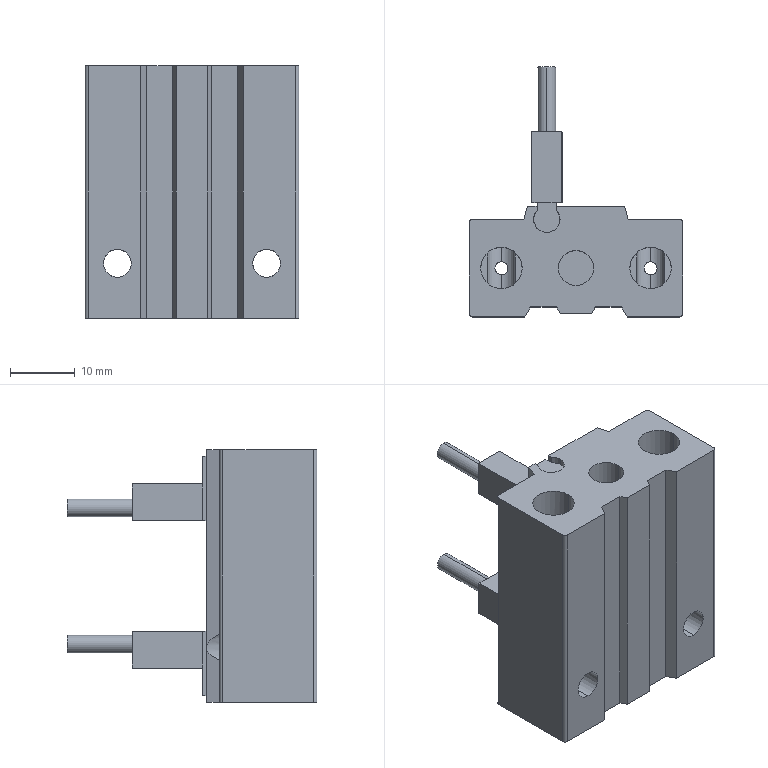Part | STEP file | MGJ10-20-F8NL1 | 1 solid | 127 faces | box 33 x 38.5 x 39 mm | volume 17194 mm3 | plane 60 | cylinder 47 | cone 20 | commonest cylinder face diameters 3.24 x8 4 x6 1 x4 2 x4 2.46 x4 2.7 x4